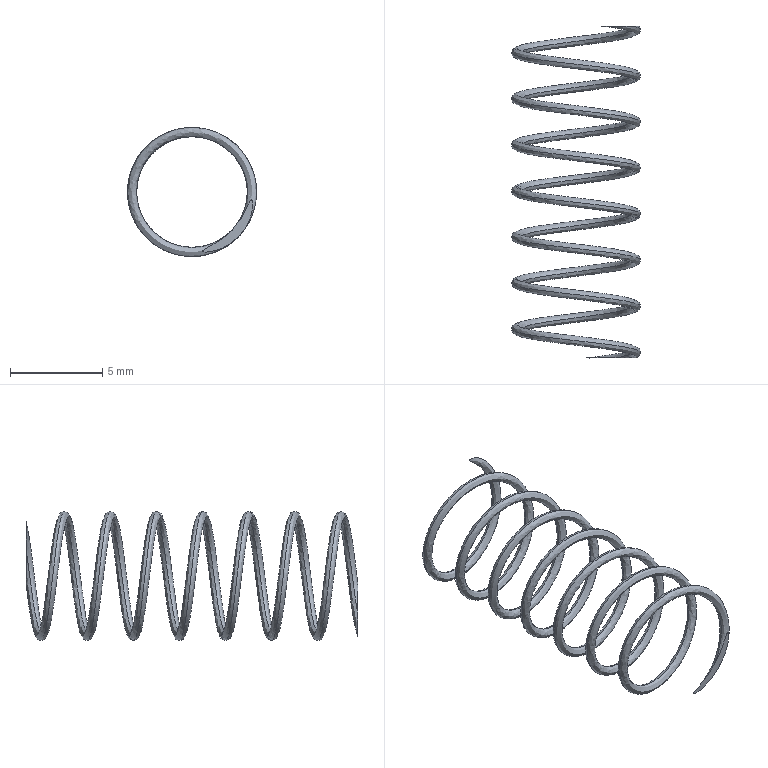Part | SolidWorks | features Helix 1, ICE 1, RefAxis 1, Sweep 1 | 1 solid | 4 faces | box 7 x 18 x 7 mm | volume 28.721 mm3 | spline 2 | plane 2